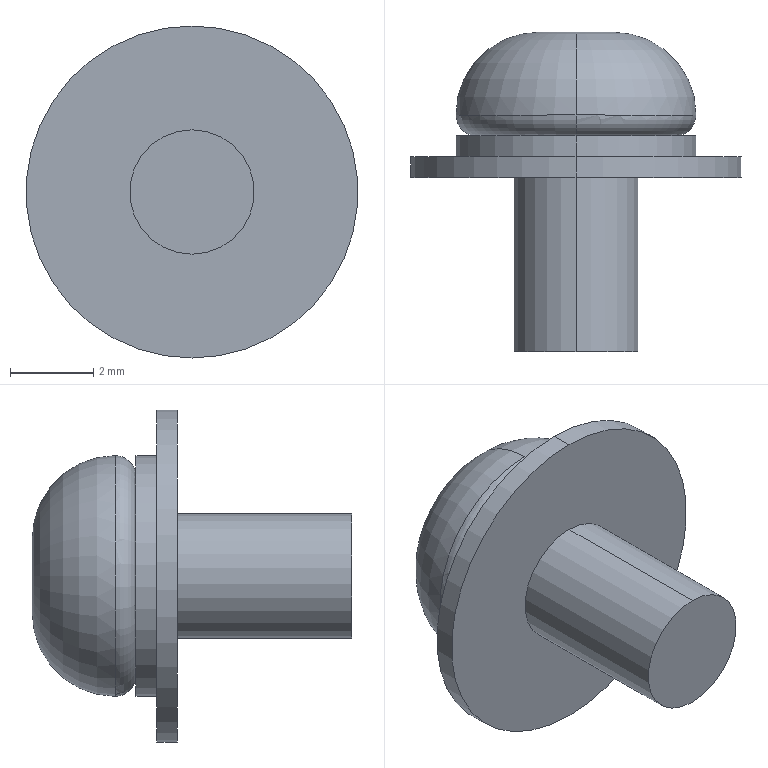Part | SolidWorks | features RefAxis 6, 3DProfileFeature 2, Revolution 1 | 1 solid | 15 faces | box 8 x 7.7 x 8 mm | volume 119.911 mm3 | cylinder 6 | plane 5 | torus 4 | commonest cylinder face diameters 3 x2 5.8 x2 8 x2
STEP:
#1=CARTESIAN_POINT('',(0.,3.5,-0.9));
#2=VERTEX_POINT('',#1);
#3=CARTESIAN_POINT('',(0.,3.5,0.9));
#4=VERTEX_POINT('',#3);
#5=CARTESIAN_POINT('',(0.,3.5,0.));
#6=DIRECTION('',(0.,-1.,0.));
#7=DIRECTION('',(0.,0.,-1.));
#8=AXIS2_PLACEMENT_3D('',#5,#6,#7);
#9=CIRCLE('',#8,0.9);
#10=EDGE_CURVE('',#2,#4,#9,.T.);
#11=ORIENTED_EDGE('',*,*,#10,.T.);
#12=CARTESIAN_POINT('',(0.,1.5,2.9));
#13=VERTEX_POINT('',#12);
#14=CARTESIAN_POINT('',(0.,1.5,0.9));
#15=DIRECTION('',(1.,0.,0.));
#16=DIRECTION('',(0.,0.,-1.));
#17=AXIS2_PLACEMENT_3D('',#14,#15,#16);
#18=CIRCLE('',#17,2.);
#19=EDGE_CURVE('',#4,#13,#18,.T.);
#20=ORIENTED_EDGE('',*,*,#19,.T.);
#21=CARTESIAN_POINT('',(0.,1.5,-2.9));
#22=VERTEX_POINT('',#21);
#23=CARTESIAN_POINT('',(0.,1.5,0.));
#24=DIRECTION('',(0.,-1.,0.));
#25=DIRECTION('',(0.,0.,-1.));
#26=AXIS2_PLACEMENT_3D('',#23,#24,#25);
#27=CIRCLE('',#26,2.9);
#28=EDGE_CURVE('',#22,#13,#27,.T.);
#29=ORIENTED_EDGE('',*,*,#28,.F.);
#30=CARTESIAN_POINT('',(0.,1.5,-0.9));
#31=DIRECTION('',(-1.,0.,0.));
#32=DIRECTION('',(0.,0.,1.));
#33=AXIS2_PLACEMENT_3D('',#30,#31,#32);
#34=CIRCLE('',#33,2.);
#35=EDGE_CURVE('',#2,#22,#34,.T.);
#36=ORIENTED_EDGE('',*,*,#35,.F.);
#37=EDGE_LOOP('',(#11,#20,#29,#36));
#38=FACE_OUTER_BOUND('',#37,.T.);
#39=CARTESIAN_POINT('',(0.,1.5,0.));
#40=DIRECTION('',(0.,-1.,0.));
#41=DIRECTION('',(0.,0.,-1.));
#42=AXIS2_PLACEMENT_3D('',#39,#40,#41);
#43=TOROIDAL_SURFACE('',#42,0.9,2.);
#44=ADVANCED_FACE('',(#38),#43,.T.);
#45=ORIENTED_EDGE('',*,*,#28,.T.);
#46=CARTESIAN_POINT('',(0.,1.,2.4));
#47=VERTEX_POINT('',#46);
#48=CARTESIAN_POINT('',(0.,1.5,2.4));
#49=DIRECTION('',(1.,0.,0.));
#50=DIRECTION('',(0.,0.,-1.));
#51=AXIS2_PLACEMENT_3D('',#48,#49,#50);
#52=CIRCLE('',#51,0.5);
#53=EDGE_CURVE('',#13,#47,#52,.T.);
#54=ORIENTED_EDGE('',*,*,#53,.T.);
#55=CARTESIAN_POINT('',(0.,1.,-2.4));
#56=VERTEX_POINT('',#55);
#57=CARTESIAN_POINT('',(0.,1.,0.));
#58=DIRECTION('',(0.,-1.,0.));
#59=DIRECTION('',(0.,0.,-1.));
#60=AXIS2_PLACEMENT_3D('',#57,#58,#59);
#61=CIRCLE('',#60,2.4);
#62=EDGE_CURVE('',#56,#47,#61,.T.);
#63=ORIENTED_EDGE('',*,*,#62,.F.);
#64=CARTESIAN_POINT('',(0.,1.5,-2.4));
#65=DIRECTION('',(-1.,0.,0.));
#66=DIRECTION('',(0.,0.,1.));
#67=AXIS2_PLACEMENT_3D('',#64,#65,#66);
#68=CIRCLE('',#67,0.5);
#69=EDGE_CURVE('',#22,#56,#68,.T.);
#70=ORIENTED_EDGE('',*,*,#69,.F.);
#71=EDGE_LOOP('',(#45,#54,#63,#70));
#72=FACE_OUTER_BOUND('',#71,.T.);
#73=CARTESIAN_POINT('',(0.,1.5,0.));
#74=DIRECTION('',(0.,-1.,0.));
#75=DIRECTION('',(0.,0.,-1.));
#76=AXIS2_PLACEMENT_3D('',#73,#74,#75);
#77=TOROIDAL_SURFACE('',#76,2.4,0.5);
#78=ADVANCED_FACE('',(#72),#77,.T.);
#79=CARTESIAN_POINT('',(0.,1.,-2.9));
#80=VERTEX_POINT('',#79);
#81=CARTESIAN_POINT('',(0.,1.,2.9));
#82=VERTEX_POINT('',#81);
#83=CARTESIAN_POINT('',(0.,1.,0.));
#84=DIRECTION('',(0.,-1.,0.));
#85=DIRECTION('',(0.,0.,-1.));
#86=AXIS2_PLACEMENT_3D('',#83,#84,#85);
#87=CIRCLE('',#86,2.9);
#88=EDGE_CURVE('',#80,#82,#87,.T.);
#89=ORIENTED_EDGE('',*,*,#88,.T.);
#90=CARTESIAN_POINT('',(0.,0.5,2.9));
#91=VERTEX_POINT('',#90);
#92=CARTESIAN_POINT('',(0.,3.5,2.9));
#93=DIRECTION('',(0.,-1.,0.));
#94=VECTOR('',#93,1000.);
#95=LINE('',#92,#94);
#96=EDGE_CURVE('',#82,#91,#95,.T.);
#97=ORIENTED_EDGE('',*,*,#96,.T.);
#98=CARTESIAN_POINT('',(0.,0.5,-2.9));
#99=VERTEX_POINT('',#98);
#100=CARTESIAN_POINT('',(0.,0.5,0.));
#101=DIRECTION('',(0.,-1.,0.));
#102=DIRECTION('',(0.,0.,-1.));
#103=AXIS2_PLACEMENT_3D('',#100,#101,#102);
#104=CIRCLE('',#103,2.9);
#105=EDGE_CURVE('',#99,#91,#104,.T.);
#106=ORIENTED_EDGE('',*,*,#105,.F.);
#107=CARTESIAN_POINT('',(0.,3.5,-2.9));
#108=DIRECTION('',(0.,-1.,0.));
#109=VECTOR('',#108,1000.);
#110=LINE('',#107,#109);
#111=EDGE_CURVE('',#80,#99,#110,.T.);
#112=ORIENTED_EDGE('',*,*,#111,.F.);
#113=EDGE_LOOP('',(#89,#97,#106,#112));
#114=FACE_OUTER_BOUND('',#113,.T.);
#115=CARTESIAN_POINT('',(0.,3.5,0.));
#116=DIRECTION('',(0.,-1.,0.));
#117=DIRECTION('',(0.,0.,-1.));
#118=AXIS2_PLACEMENT_3D('',#115,#116,#117);
#119=CYLINDRICAL_SURFACE('',#118,2.9);
#120=ADVANCED_FACE('',(#114),#119,.T.);
#121=CARTESIAN_POINT('',(0.,0.5,-4.));
#122=VERTEX_POINT('',#121);
#123=CARTESIAN_POINT('',(0.,0.5,4.));
#124=VERTEX_POINT('',#123);
#125=CARTESIAN_POINT('',(0.,0.5,0.));
#126=DIRECTION('',(0.,-1.,0.));
#127=DIRECTION('',(0.,0.,-1.));
#128=AXIS2_PLACEMENT_3D('',#125,#126,#127);
#129=CIRCLE('',#128,4.);
#130=EDGE_CURVE('',#122,#124,#129,.T.);
#131=ORIENTED_EDGE('',*,*,#130,.T.);
#132=CARTESIAN_POINT('',(0.,0.,4.));
#133=VERTEX_POINT('',#132);
#134=CARTESIAN_POINT('',(0.,3.5,4.));
#135=DIRECTION('',(0.,-1.,0.));
#136=VECTOR('',#135,1000.);
#137=LINE('',#134,#136);
#138=EDGE_CURVE('',#124,#133,#137,.T.);
#139=ORIENTED_EDGE('',*,*,#138,.T.);
#140=CARTESIAN_POINT('',(0.,0.,-4.));
#141=VERTEX_POINT('',#140);
#142=CARTESIAN_POINT('',(0.,0.,0.));
#143=DIRECTION('',(0.,-1.,0.));
#144=DIRECTION('',(0.,0.,-1.));
#145=AXIS2_PLACEMENT_3D('',#142,#143,#144);
#146=CIRCLE('',#145,4.);
#147=EDGE_CURVE('',#141,#133,#146,.T.);
#148=ORIENTED_EDGE('',*,*,#147,.F.);
#149=CARTESIAN_POINT('',(0.,3.5,-4.));
#150=DIRECTION('',(0.,-1.,0.));
#151=VECTOR('',#150,1000.);
#152=LINE('',#149,#151);
#153=EDGE_CURVE('',#122,#141,#152,.T.);
#154=ORIENTED_EDGE('',*,*,#153,.F.);
#155=EDGE_LOOP('',(#131,#139,#148,#154));
#156=FACE_OUTER_BOUND('',#155,.T.);
#157=CARTESIAN_POINT('',(0.,3.5,0.));
#158=DIRECTION('',(0.,-1.,0.));
#159=DIRECTION('',(0.,0.,-1.));
#160=AXIS2_PLACEMENT_3D('',#157,#158,#159);
#161=CYLINDRICAL_SURFACE('',#160,4.);
#162=ADVANCED_FACE('',(#156),#161,.T.);
#163=CARTESIAN_POINT('',(0.,0.,-1.5));
#164=VERTEX_POINT('',#163);
#165=CARTESIAN_POINT('',(0.,0.,1.5));
#166=VERTEX_POINT('',#165);
#167=CARTESIAN_POINT('',(0.,0.,0.));
#168=DIRECTION('',(0.,-1.,0.));
#169=DIRECTION('',(0.,0.,-1.));
#170=AXIS2_PLACEMENT_3D('',#167,#168,#169);
#171=CIRCLE('',#170,1.5);
#172=EDGE_CURVE('',#164,#166,#171,.T.);
#173=ORIENTED_EDGE('',*,*,#172,.T.);
#174=CARTESIAN_POINT('',(0.,-4.2,1.5));
#175=VERTEX_POINT('',#174);
#176=CARTESIAN_POINT('',(0.,3.5,1.5));
#177=DIRECTION('',(0.,-1.,0.));
#178=VECTOR('',#177,1000.);
#179=LINE('',#176,#178);
#180=EDGE_CURVE('',#166,#175,#179,.T.);
#181=ORIENTED_EDGE('',*,*,#180,.T.);
#182=CARTESIAN_POINT('',(0.,-4.2,-1.5));
#183=VERTEX_POINT('',#182);
#184=CARTESIAN_POINT('',(0.,-4.2,0.));
#185=DIRECTION('',(0.,-1.,0.));
#186=DIRECTION('',(0.,0.,-1.));
#187=AXIS2_PLACEMENT_3D('',#184,#185,#186);
#188=CIRCLE('',#187,1.5);
#189=EDGE_CURVE('',#183,#175,#188,.T.);
#190=ORIENTED_EDGE('',*,*,#189,.F.);
#191=CARTESIAN_POINT('',(0.,3.5,-1.5));
#192=DIRECTION('',(0.,-1.,0.));
#193=VECTOR('',#192,1000.);
#194=LINE('',#191,#193);
#195=EDGE_CURVE('',#164,#183,#194,.T.);
#196=ORIENTED_EDGE('',*,*,#195,.F.);
#197=EDGE_LOOP('',(#173,#181,#190,#196));
#198=FACE_OUTER_BOUND('',#197,.T.);
#199=CARTESIAN_POINT('',(0.,3.5,0.));
#200=DIRECTION('',(0.,-1.,0.));
#201=DIRECTION('',(0.,0.,-1.));
#202=AXIS2_PLACEMENT_3D('',#199,#200,#201);
#203=CYLINDRICAL_SURFACE('',#202,1.5);
#204=ADVANCED_FACE('',(#198),#203,.T.);
#205=ORIENTED_EDGE('',*,*,#189,.T.);
#206=CARTESIAN_POINT('',(0.,-4.2,0.));
#207=DIRECTION('',(0.,-1.,0.));
#208=DIRECTION('',(0.,0.,-1.));
#209=AXIS2_PLACEMENT_3D('',#206,#207,#208);
#210=CIRCLE('',#209,1.5);
#211=EDGE_CURVE('',#175,#183,#210,.T.);
#212=ORIENTED_EDGE('',*,*,#211,.T.);
#213=EDGE_LOOP('',(#205,#212));
#214=FACE_OUTER_BOUND('',#213,.T.);
#215=CARTESIAN_POINT('',(0.,-4.2,0.));
#216=DIRECTION('',(0.,1.,0.));
#217=DIRECTION('',(0.,0.,1.));
#218=AXIS2_PLACEMENT_3D('',#215,#216,#217);
#219=PLANE('',#218);
#220=ADVANCED_FACE('',(#214),#219,.F.);
#221=ORIENTED_EDGE('',*,*,#180,.F.);
#222=CARTESIAN_POINT('',(0.,0.,0.));
#223=DIRECTION('',(0.,-1.,0.));
#224=DIRECTION('',(0.,0.,-1.));
#225=AXIS2_PLACEMENT_3D('',#222,#223,#224);
#226=CIRCLE('',#225,1.5);
#227=EDGE_CURVE('',#166,#164,#226,.T.);
#228=ORIENTED_EDGE('',*,*,#227,.T.);
#229=ORIENTED_EDGE('',*,*,#195,.T.);
#230=ORIENTED_EDGE('',*,*,#211,.F.);
#231=EDGE_LOOP('',(#221,#228,#229,#230));
#232=FACE_OUTER_BOUND('',#231,.T.);
#233=CARTESIAN_POINT('',(0.,3.5,0.));
#234=DIRECTION('',(0.,-1.,0.));
#235=DIRECTION('',(0.,0.,-1.));
#236=AXIS2_PLACEMENT_3D('',#233,#234,#235);
#237=CYLINDRICAL_SURFACE('',#236,1.5);
#238=ADVANCED_FACE('',(#232),#237,.T.);
#239=ORIENTED_EDGE('',*,*,#172,.F.);
#240=ORIENTED_EDGE('',*,*,#227,.F.);
#241=EDGE_LOOP('',(#239,#240));
#242=FACE_BOUND('',#241,.T.);
#243=ORIENTED_EDGE('',*,*,#147,.T.);
#244=CARTESIAN_POINT('',(0.,0.,0.));
#245=DIRECTION('',(0.,-1.,0.));
#246=DIRECTION('',(0.,0.,-1.));
#247=AXIS2_PLACEMENT_3D('',#244,#245,#246);
#248=CIRCLE('',#247,4.);
#249=EDGE_CURVE('',#133,#141,#248,.T.);
#250=ORIENTED_EDGE('',*,*,#249,.T.);
#251=EDGE_LOOP('',(#243,#250));
#252=FACE_OUTER_BOUND('',#251,.T.);
#253=CARTESIAN_POINT('',(0.,0.,1.5));
#254=DIRECTION('',(0.,1.,0.));
#255=DIRECTION('',(0.,0.,1.));
#256=AXIS2_PLACEMENT_3D('',#253,#254,#255);
#257=PLANE('',#256);
#258=ADVANCED_FACE('',(#242,#252),#257,.F.);
#259=ORIENTED_EDGE('',*,*,#138,.F.);
#260=CARTESIAN_POINT('',(0.,0.5,0.));
#261=DIRECTION('',(0.,-1.,0.));
#262=DIRECTION('',(0.,0.,-1.));
#263=AXIS2_PLACEMENT_3D('',#260,#261,#262);
#264=CIRCLE('',#263,4.);
#265=EDGE_CURVE('',#124,#122,#264,.T.);
#266=ORIENTED_EDGE('',*,*,#265,.T.);
#267=ORIENTED_EDGE('',*,*,#153,.T.);
#268=ORIENTED_EDGE('',*,*,#249,.F.);
#269=EDGE_LOOP('',(#259,#266,#267,#268));
#270=FACE_OUTER_BOUND('',#269,.T.);
#271=CARTESIAN_POINT('',(0.,3.5,0.));
#272=DIRECTION('',(0.,-1.,0.));
#273=DIRECTION('',(0.,0.,-1.));
#274=AXIS2_PLACEMENT_3D('',#271,#272,#273);
#275=CYLINDRICAL_SURFACE('',#274,4.);
#276=ADVANCED_FACE('',(#270),#275,.T.);
#277=ORIENTED_EDGE('',*,*,#130,.F.);
#278=ORIENTED_EDGE('',*,*,#265,.F.);
#279=EDGE_LOOP('',(#277,#278));
#280=FACE_OUTER_BOUND('',#279,.T.);
#281=ORIENTED_EDGE('',*,*,#105,.T.);
#282=CARTESIAN_POINT('',(0.,0.5,0.));
#283=DIRECTION('',(0.,-1.,0.));
#284=DIRECTION('',(0.,0.,-1.));
#285=AXIS2_PLACEMENT_3D('',#282,#283,#284);
#286=CIRCLE('',#285,2.9);
#287=EDGE_CURVE('',#91,#99,#286,.T.);
#288=ORIENTED_EDGE('',*,*,#287,.T.);
#289=EDGE_LOOP('',(#281,#288));
#290=FACE_BOUND('',#289,.T.);
#291=CARTESIAN_POINT('',(0.,0.5,4.));
#292=DIRECTION('',(0.,-1.,0.));
#293=DIRECTION('',(0.,0.,-1.));
#294=AXIS2_PLACEMENT_3D('',#291,#292,#293);
#295=PLANE('',#294);
#296=ADVANCED_FACE('',(#280,#290),#295,.F.);
#297=ORIENTED_EDGE('',*,*,#96,.F.);
#298=CARTESIAN_POINT('',(0.,1.,0.));
#299=DIRECTION('',(0.,-1.,0.));
#300=DIRECTION('',(0.,0.,-1.));
#301=AXIS2_PLACEMENT_3D('',#298,#299,#300);
#302=CIRCLE('',#301,2.9);
#303=EDGE_CURVE('',#82,#80,#302,.T.);
#304=ORIENTED_EDGE('',*,*,#303,.T.);
#305=ORIENTED_EDGE('',*,*,#111,.T.);
#306=ORIENTED_EDGE('',*,*,#287,.F.);
#307=EDGE_LOOP('',(#297,#304,#305,#306));
#308=FACE_OUTER_BOUND('',#307,.T.);
#309=CARTESIAN_POINT('',(0.,3.5,0.));
#310=DIRECTION('',(0.,-1.,0.));
#311=DIRECTION('',(0.,0.,-1.));
#312=AXIS2_PLACEMENT_3D('',#309,#310,#311);
#313=CYLINDRICAL_SURFACE('',#312,2.9);
#314=ADVANCED_FACE('',(#308),#313,.T.);
#315=ORIENTED_EDGE('',*,*,#88,.F.);
#316=ORIENTED_EDGE('',*,*,#303,.F.);
#317=EDGE_LOOP('',(#315,#316));
#318=FACE_OUTER_BOUND('',#317,.T.);
#319=ORIENTED_EDGE('',*,*,#62,.T.);
#320=CARTESIAN_POINT('',(0.,1.,0.));
#321=DIRECTION('',(0.,-1.,0.));
#322=DIRECTION('',(0.,0.,-1.));
#323=AXIS2_PLACEMENT_3D('',#320,#321,#322);
#324=CIRCLE('',#323,2.4);
#325=EDGE_CURVE('',#47,#56,#324,.T.);
#326=ORIENTED_EDGE('',*,*,#325,.T.);
#327=EDGE_LOOP('',(#319,#326));
#328=FACE_BOUND('',#327,.T.);
#329=CARTESIAN_POINT('',(0.,1.,2.9));
#330=DIRECTION('',(0.,-1.,0.));
#331=DIRECTION('',(0.,0.,-1.));
#332=AXIS2_PLACEMENT_3D('',#329,#330,#331);
#333=PLANE('',#332);
#334=ADVANCED_FACE('',(#318,#328),#333,.F.);
#335=ORIENTED_EDGE('',*,*,#53,.F.);
#336=CARTESIAN_POINT('',(0.,1.5,0.));
#337=DIRECTION('',(0.,-1.,0.));
#338=DIRECTION('',(0.,0.,-1.));
#339=AXIS2_PLACEMENT_3D('',#336,#337,#338);
#340=CIRCLE('',#339,2.9);
#341=EDGE_CURVE('',#13,#22,#340,.T.);
#342=ORIENTED_EDGE('',*,*,#341,.T.);
#343=ORIENTED_EDGE('',*,*,#69,.T.);
#344=ORIENTED_EDGE('',*,*,#325,.F.);
#345=EDGE_LOOP('',(#335,#342,#343,#344));
#346=FACE_OUTER_BOUND('',#345,.T.);
#347=CARTESIAN_POINT('',(0.,1.5,0.));
#348=DIRECTION('',(0.,-1.,0.));
#349=DIRECTION('',(0.,0.,-1.));
#350=AXIS2_PLACEMENT_3D('',#347,#348,#349);
#351=TOROIDAL_SURFACE('',#350,2.4,0.5);
#352=ADVANCED_FACE('',(#346),#351,.T.);
#353=ORIENTED_EDGE('',*,*,#19,.F.);
#354=CARTESIAN_POINT('',(0.,3.5,0.));
#355=DIRECTION('',(0.,-1.,0.));
#356=DIRECTION('',(0.,0.,-1.));
#357=AXIS2_PLACEMENT_3D('',#354,#355,#356);
#358=CIRCLE('',#357,0.9);
#359=EDGE_CURVE('',#4,#2,#358,.T.);
#360=ORIENTED_EDGE('',*,*,#359,.T.);
#361=ORIENTED_EDGE('',*,*,#35,.T.);
#362=ORIENTED_EDGE('',*,*,#341,.F.);
#363=EDGE_LOOP('',(#353,#360,#361,#362));
#364=FACE_OUTER_BOUND('',#363,.T.);
#365=CARTESIAN_POINT('',(0.,1.5,0.));
#366=DIRECTION('',(0.,-1.,0.));
#367=DIRECTION('',(0.,0.,-1.));
#368=AXIS2_PLACEMENT_3D('',#365,#366,#367);
#369=TOROIDAL_SURFACE('',#368,0.9,2.);
#370=ADVANCED_FACE('',(#364),#369,.T.);
#371=ORIENTED_EDGE('',*,*,#10,.F.);
#372=ORIENTED_EDGE('',*,*,#359,.F.);
#373=EDGE_LOOP('',(#371,#372));
#374=FACE_OUTER_BOUND('',#373,.T.);
#375=CARTESIAN_POINT('',(0.,3.5,0.9));
#376=DIRECTION('',(0.,-1.,0.));
#377=DIRECTION('',(0.,0.,-1.));
#378=AXIS2_PLACEMENT_3D('',#375,#376,#377);
#379=PLANE('',#378);
#380=ADVANCED_FACE('',(#374),#379,.F.);
#381=CLOSED_SHELL('',(#44,#78,#120,#162,#204,#220,#238,#258,#276,#296,#314,#334,#352,#370,#380));
#382=MANIFOLD_SOLID_BREP('',#381);
#383=CARTESIAN_POINT('',(0.,0.,0.));
#384=DIRECTION('',(0.,0.,1.));
#385=DIRECTION('',(1.,0.,0.));
#386=AXIS2_PLACEMENT_3D('',#383,#384,#385);
#387=(LENGTH_UNIT()NAMED_UNIT(*)SI_UNIT(.MILLI.,.METRE.));
#388=UNCERTAINTY_MEASURE_WITH_UNIT(LENGTH_MEASURE(0.00001),#387,'','');
#389=(NAMED_UNIT(*)PLANE_ANGLE_UNIT()SI_UNIT($,.RADIAN.));
#390=(NAMED_UNIT(*)SI_UNIT($,.STERADIAN.)SOLID_ANGLE_UNIT());
#391=(GEOMETRIC_REPRESENTATION_CONTEXT(3)GLOBAL_UNCERTAINTY_ASSIGNED_CONTEXT((#388))GLOBAL_UNIT_ASSIGNED_CONTEXT((#387,#389,#390))REPRESENTATION_CONTEXT('',''));
#392=ADVANCED_BREP_SHAPE_REPRESENTATION('',(#382,#386),#391);